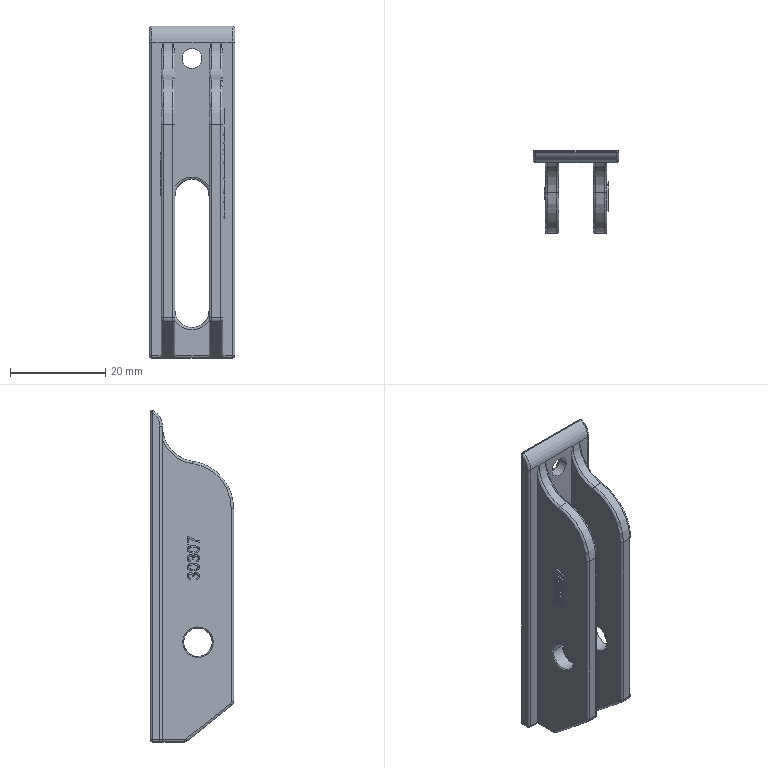Part | STEP file | 101000007593 | 1 solid | 256 faces | box 18 x 17.5 x 69.846 mm | volume 7199 mm3 | plane 132 | cylinder 55 | spline 37 | torus 24 | cone 4 | sphere 4 | commonest cylinder face diameters 1 x24 2 x4 6 x4 0.204 x2 0.206 x2 0.257 x2